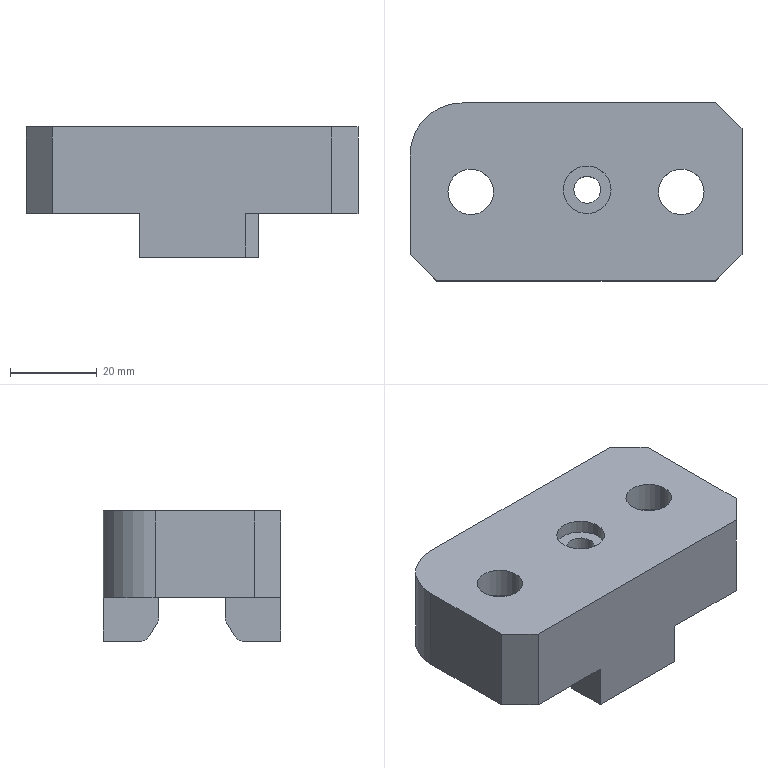Part | STEP file | lll_id2726_x_t | 1 solid | 35 faces | box 76.5 x 41 x 30 mm | volume 58200 mm3 | plane 24 | cylinder 11 | commonest cylinder face diameters 4 x4 10.5 x2 19.007 x2 6.2 x1 11 x1 24 x1
STEP:
#1=CARTESIAN_POINT('',(3745.164,7.62,-2.113));
#2=VERTEX_POINT('',#1);
#3=CARTESIAN_POINT('',(3772.5,7.62,-2.113));
#4=VERTEX_POINT('',#3);
#5=CARTESIAN_POINT('',(3772.5,7.62,-2.113));
#6=DIRECTION('',(1.,0.,0.));
#7=VECTOR('',#6,1.);
#8=LINE('',#5,#7);
#9=EDGE_CURVE('',#2,#4,#8,.T.);
#10=ORIENTED_EDGE('',*,*,#9,.F.);
#11=CARTESIAN_POINT('',(3745.164,7.905,-3.142));
#12=VERTEX_POINT('',#11);
#13=CARTESIAN_POINT('',(3745.164,9.62,-2.113));
#14=DIRECTION('',(1.,0.,0.));
#15=DIRECTION('',(0.,0.,-1.));
#16=AXIS2_PLACEMENT_3D('',#13,#14,#15);
#17=CIRCLE('',#16,2.);
#18=EDGE_CURVE('',#2,#12,#17,.T.);
#19=ORIENTED_EDGE('',*,*,#18,.T.);
#20=CARTESIAN_POINT('',(3772.5,7.905,-3.142));
#21=VERTEX_POINT('',#20);
#22=CARTESIAN_POINT('',(3758.811,7.905,-3.142));
#23=DIRECTION('',(-1.,0.,0.));
#24=VECTOR('',#23,1.);
#25=LINE('',#22,#24);
#26=EDGE_CURVE('',#21,#12,#25,.T.);
#27=ORIENTED_EDGE('',*,*,#26,.F.);
#28=CARTESIAN_POINT('',(3772.5,9.62,-2.113));
#29=DIRECTION('',(1.,0.,0.));
#30=DIRECTION('',(0.,0.,-1.));
#31=AXIS2_PLACEMENT_3D('',#28,#29,#30);
#32=CIRCLE('',#31,2.);
#33=EDGE_CURVE('',#4,#21,#32,.T.);
#34=ORIENTED_EDGE('',*,*,#33,.F.);
#35=EDGE_LOOP('',(#10,#19,#27,#34));
#36=FACE_OUTER_BOUND('',#35,.T.);
#37=CARTESIAN_POINT('',(3831.,9.62,-2.113));
#38=DIRECTION('',(1.,0.,0.));
#39=DIRECTION('',(0.,1.,0.));
#40=AXIS2_PLACEMENT_3D('',#37,#38,#39);
#41=CYLINDRICAL_SURFACE('',#40,2.);
#42=ADVANCED_FACE('',(#36),#41,.T.);
#43=CARTESIAN_POINT('',(3745.164,-7.62,-2.113));
#44=VERTEX_POINT('',#43);
#45=CARTESIAN_POINT('',(3745.164,-7.905,-3.142));
#46=VERTEX_POINT('',#45);
#47=CARTESIAN_POINT('',(3745.164,-9.62,-2.113));
#48=DIRECTION('',(-1.,0.,0.));
#49=DIRECTION('',(0.,0.,-1.));
#50=AXIS2_PLACEMENT_3D('',#47,#48,#49);
#51=CIRCLE('',#50,2.);
#52=EDGE_CURVE('',#44,#46,#51,.T.);
#53=ORIENTED_EDGE('',*,*,#52,.F.);
#54=CARTESIAN_POINT('',(3772.5,-7.62,-2.113));
#55=VERTEX_POINT('',#54);
#56=CARTESIAN_POINT('',(3758.811,-7.62,-2.113));
#57=DIRECTION('',(-1.,0.,0.));
#58=VECTOR('',#57,1.);
#59=LINE('',#56,#58);
#60=EDGE_CURVE('',#55,#44,#59,.T.);
#61=ORIENTED_EDGE('',*,*,#60,.F.);
#62=CARTESIAN_POINT('',(3772.5,-7.905,-3.142));
#63=VERTEX_POINT('',#62);
#64=CARTESIAN_POINT('',(3772.5,-9.62,-2.113));
#65=DIRECTION('',(1.,0.,0.));
#66=DIRECTION('',(0.,0.,-1.));
#67=AXIS2_PLACEMENT_3D('',#64,#65,#66);
#68=CIRCLE('',#67,2.);
#69=EDGE_CURVE('',#63,#55,#68,.T.);
#70=ORIENTED_EDGE('',*,*,#69,.F.);
#71=CARTESIAN_POINT('',(3772.5,-7.905,-3.142));
#72=DIRECTION('',(1.,0.,0.));
#73=VECTOR('',#72,1.);
#74=LINE('',#71,#73);
#75=EDGE_CURVE('',#46,#63,#74,.T.);
#76=ORIENTED_EDGE('',*,*,#75,.F.);
#77=EDGE_LOOP('',(#53,#61,#70,#76));
#78=FACE_OUTER_BOUND('',#77,.T.);
#79=CARTESIAN_POINT('',(3831.,-9.62,-2.113));
#80=DIRECTION('',(-1.,0.,0.));
#81=DIRECTION('',(0.,-1.,0.));
#82=AXIS2_PLACEMENT_3D('',#79,#80,#81);
#83=CYLINDRICAL_SURFACE('',#82,2.);
#84=ADVANCED_FACE('',(#78),#83,.T.);
#85=CARTESIAN_POINT('',(3772.5,-9.937,-6.529));
#86=VERTEX_POINT('',#85);
#87=CARTESIAN_POINT('',(3772.5,1.088,11.847));
#88=DIRECTION('',(0.,0.5145,0.8575));
#89=VECTOR('',#88,1.);
#90=LINE('',#87,#89);
#91=EDGE_CURVE('',#86,#63,#90,.T.);
#92=ORIENTED_EDGE('',*,*,#91,.T.);
#93=ORIENTED_EDGE('',*,*,#69,.T.);
#94=CARTESIAN_POINT('',(3772.5,-7.62,2.5));
#95=VERTEX_POINT('',#94);
#96=CARTESIAN_POINT('',(3772.5,-7.62,12.5));
#97=DIRECTION('',(0.,0.,-1.));
#98=VECTOR('',#97,1.);
#99=LINE('',#96,#98);
#100=EDGE_CURVE('',#95,#55,#99,.T.);
#101=ORIENTED_EDGE('',*,*,#100,.F.);
#102=CARTESIAN_POINT('',(3772.5,-17.5,2.5));
#103=VERTEX_POINT('',#102);
#104=CARTESIAN_POINT('',(3772.5,0.00007422,2.5));
#105=DIRECTION('',(0.,-1.,0.));
#106=VECTOR('',#105,1.);
#107=LINE('',#104,#106);
#108=EDGE_CURVE('',#95,#103,#107,.T.);
#109=ORIENTED_EDGE('',*,*,#108,.T.);
#110=CARTESIAN_POINT('',(3772.5,-17.5,-7.5));
#111=VERTEX_POINT('',#110);
#112=CARTESIAN_POINT('',(3772.5,-17.5,-7.5));
#113=DIRECTION('',(0.,0.,-1.));
#114=VECTOR('',#113,1.);
#115=LINE('',#112,#114);
#116=EDGE_CURVE('',#103,#111,#115,.T.);
#117=ORIENTED_EDGE('',*,*,#116,.T.);
#118=CARTESIAN_POINT('',(3772.5,-11.652,-7.5));
#119=VERTEX_POINT('',#118);
#120=CARTESIAN_POINT('',(3772.5,1.,-7.5));
#121=DIRECTION('',(0.,1.,0.));
#122=VECTOR('',#121,1.);
#123=LINE('',#120,#122);
#124=EDGE_CURVE('',#111,#119,#123,.T.);
#125=ORIENTED_EDGE('',*,*,#124,.T.);
#126=CARTESIAN_POINT('',(3772.5,-11.652,-5.5));
#127=DIRECTION('',(1.,0.,0.));
#128=DIRECTION('',(0.,0.,-1.));
#129=AXIS2_PLACEMENT_3D('',#126,#127,#128);
#130=CIRCLE('',#129,2.);
#131=EDGE_CURVE('',#119,#86,#130,.T.);
#132=ORIENTED_EDGE('',*,*,#131,.T.);
#133=EDGE_LOOP('',(#92,#93,#101,#109,#117,#125,#132));
#134=FACE_OUTER_BOUND('',#133,.T.);
#135=CARTESIAN_POINT('',(3772.5,0.00007422,12.5));
#136=DIRECTION('',(1.,0.,0.));
#137=DIRECTION('',(0.,0.,-1.));
#138=AXIS2_PLACEMENT_3D('',#135,#136,#137);
#139=PLANE('',#138);
#140=ADVANCED_FACE('',(#134),#139,.T.);
#141=CARTESIAN_POINT('',(3772.5,7.62,2.5));
#142=VERTEX_POINT('',#141);
#143=CARTESIAN_POINT('',(3772.5,7.62,12.5));
#144=DIRECTION('',(0.,0.,-1.));
#145=VECTOR('',#144,1.);
#146=LINE('',#143,#145);
#147=EDGE_CURVE('',#142,#4,#146,.T.);
#148=ORIENTED_EDGE('',*,*,#147,.T.);
#149=ORIENTED_EDGE('',*,*,#33,.T.);
#150=CARTESIAN_POINT('',(3772.5,9.937,-6.529));
#151=VERTEX_POINT('',#150);
#152=CARTESIAN_POINT('',(3772.5,-1.088,11.847));
#153=DIRECTION('',(0.,0.5145,-0.8575));
#154=VECTOR('',#153,1.);
#155=LINE('',#152,#154);
#156=EDGE_CURVE('',#21,#151,#155,.T.);
#157=ORIENTED_EDGE('',*,*,#156,.T.);
#158=CARTESIAN_POINT('',(3772.5,11.652,-7.5));
#159=VERTEX_POINT('',#158);
#160=CARTESIAN_POINT('',(3772.5,11.652,-5.5));
#161=DIRECTION('',(1.,0.,0.));
#162=DIRECTION('',(0.,0.,-1.));
#163=AXIS2_PLACEMENT_3D('',#160,#161,#162);
#164=CIRCLE('',#163,2.);
#165=EDGE_CURVE('',#151,#159,#164,.T.);
#166=ORIENTED_EDGE('',*,*,#165,.T.);
#167=CARTESIAN_POINT('',(3772.5,17.5,-7.5));
#168=VERTEX_POINT('',#167);
#169=CARTESIAN_POINT('',(3772.5,-0.9999,-7.5));
#170=DIRECTION('',(0.,1.,0.));
#171=VECTOR('',#170,1.);
#172=LINE('',#169,#171);
#173=EDGE_CURVE('',#159,#168,#172,.T.);
#174=ORIENTED_EDGE('',*,*,#173,.T.);
#175=CARTESIAN_POINT('',(3772.5,17.5,2.5));
#176=VERTEX_POINT('',#175);
#177=CARTESIAN_POINT('',(3772.5,17.5,2.5));
#178=DIRECTION('',(0.,0.,1.));
#179=VECTOR('',#178,1.);
#180=LINE('',#177,#179);
#181=EDGE_CURVE('',#168,#176,#180,.T.);
#182=ORIENTED_EDGE('',*,*,#181,.T.);
#183=CARTESIAN_POINT('',(3772.5,0.00007422,2.5));
#184=DIRECTION('',(0.,-1.,0.));
#185=VECTOR('',#184,1.);
#186=LINE('',#183,#185);
#187=EDGE_CURVE('',#176,#142,#186,.T.);
#188=ORIENTED_EDGE('',*,*,#187,.T.);
#189=EDGE_LOOP('',(#148,#149,#157,#166,#174,#182,#188));
#190=FACE_OUTER_BOUND('',#189,.T.);
#191=CARTESIAN_POINT('',(3772.5,0.00007422,12.5));
#192=DIRECTION('',(1.,0.,0.));
#193=DIRECTION('',(0.,0.,-1.));
#194=AXIS2_PLACEMENT_3D('',#191,#192,#193);
#195=PLANE('',#194);
#196=ADVANCED_FACE('',(#190),#195,.T.);
#197=CARTESIAN_POINT('',(3771.997,0.00007422,15.5));
#198=VERTEX_POINT('',#197);
#199=CARTESIAN_POINT('',(3781.5,0.00007422,15.5));
#200=DIRECTION('',(0.,0.,1.));
#201=DIRECTION('',(-1.,0.,0.));
#202=AXIS2_PLACEMENT_3D('',#199,#200,#201);
#203=CIRCLE('',#202,9.504);
#204=EDGE_CURVE('',#198,#198,#203,.T.);
#205=ORIENTED_EDGE('',*,*,#204,.F.);
#206=EDGE_LOOP('',(#205));
#207=FACE_BOUND('',#206,.T.);
#208=CARTESIAN_POINT('',(3776.25,0.00007422,15.5));
#209=VERTEX_POINT('',#208);
#210=CARTESIAN_POINT('',(3781.5,0.00007422,15.5));
#211=DIRECTION('',(0.,0.,1.));
#212=DIRECTION('',(-1.,0.,0.));
#213=AXIS2_PLACEMENT_3D('',#210,#211,#212);
#214=CIRCLE('',#213,5.25);
#215=EDGE_CURVE('',#209,#209,#214,.T.);
#216=ORIENTED_EDGE('',*,*,#215,.T.);
#217=EDGE_LOOP('',(#216));
#218=FACE_BOUND('',#217,.T.);
#219=CARTESIAN_POINT('',(3781.5,0.00007422,15.5));
#220=DIRECTION('',(0.,0.,1.));
#221=DIRECTION('',(-1.,0.,0.));
#222=AXIS2_PLACEMENT_3D('',#219,#220,#221);
#223=PLANE('',#222);
#224=ADVANCED_FACE('',(#207,#218),#223,.F.);
#225=CARTESIAN_POINT('',(3775.5,7.37,2.5));
#226=VERTEX_POINT('',#225);
#227=CARTESIAN_POINT('',(3781.5,0.00007422,2.5));
#228=DIRECTION('',(0.,0.,1.));
#229=DIRECTION('',(1.,0.,0.));
#230=AXIS2_PLACEMENT_3D('',#227,#228,#229);
#231=CIRCLE('',#230,9.504);
#232=EDGE_CURVE('',#226,#226,#231,.T.);
#233=ORIENTED_EDGE('',*,*,#232,.F.);
#234=EDGE_LOOP('',(#233));
#235=FACE_BOUND('',#234,.T.);
#236=ORIENTED_EDGE('',*,*,#204,.T.);
#237=EDGE_LOOP('',(#236));
#238=FACE_BOUND('',#237,.T.);
#239=CARTESIAN_POINT('',(3781.5,0.00007422,2.5));
#240=DIRECTION('',(0.,0.,1.));
#241=DIRECTION('',(-1.,0.,0.));
#242=AXIS2_PLACEMENT_3D('',#239,#240,#241);
#243=CYLINDRICAL_SURFACE('',#242,9.504);
#244=ADVANCED_FACE('',(#235,#238),#243,.F.);
#245=CARTESIAN_POINT('',(3745.164,11.652,-7.5));
#246=VERTEX_POINT('',#245);
#247=CARTESIAN_POINT('',(3759.758,11.652,-7.5));
#248=DIRECTION('',(-1.,0.,0.));
#249=VECTOR('',#248,1.);
#250=LINE('',#247,#249);
#251=EDGE_CURVE('',#159,#246,#250,.T.);
#252=ORIENTED_EDGE('',*,*,#251,.T.);
#253=CARTESIAN_POINT('',(3745.164,20.5,-7.5));
#254=VERTEX_POINT('',#253);
#255=CARTESIAN_POINT('',(3745.164,-0.9999,-7.5));
#256=DIRECTION('',(0.,1.,0.));
#257=VECTOR('',#256,1.);
#258=LINE('',#255,#257);
#259=EDGE_CURVE('',#246,#254,#258,.T.);
#260=ORIENTED_EDGE('',*,*,#259,.T.);
#261=CARTESIAN_POINT('',(3769.5,20.5,-7.5));
#262=VERTEX_POINT('',#261);
#263=CARTESIAN_POINT('',(7344.751,20.5,-7.5));
#264=DIRECTION('',(1.,0.,0.));
#265=VECTOR('',#264,1.);
#266=LINE('',#263,#265);
#267=EDGE_CURVE('',#254,#262,#266,.T.);
#268=ORIENTED_EDGE('',*,*,#267,.T.);
#269=CARTESIAN_POINT('',(3772.5,17.5,-7.5));
#270=DIRECTION('',(0.7071,-0.7071,0.));
#271=VECTOR('',#270,1.);
#272=LINE('',#269,#271);
#273=EDGE_CURVE('',#262,#168,#272,.T.);
#274=ORIENTED_EDGE('',*,*,#273,.T.);
#275=ORIENTED_EDGE('',*,*,#173,.F.);
#276=EDGE_LOOP('',(#252,#260,#268,#274,#275));
#277=FACE_OUTER_BOUND('',#276,.T.);
#278=CARTESIAN_POINT('',(7344.751,-0.9999,-7.5));
#279=DIRECTION('',(0.,0.,1.));
#280=DIRECTION('',(1.,0.,0.));
#281=AXIS2_PLACEMENT_3D('',#278,#279,#280);
#282=PLANE('',#281);
#283=ADVANCED_FACE('',(#277),#282,.F.);
#284=CARTESIAN_POINT('',(3745.164,-20.5,-7.5));
#285=VERTEX_POINT('',#284);
#286=CARTESIAN_POINT('',(3745.164,-11.652,-7.5));
#287=VERTEX_POINT('',#286);
#288=CARTESIAN_POINT('',(3745.164,1.,-7.5));
#289=DIRECTION('',(0.,1.,0.));
#290=VECTOR('',#289,1.);
#291=LINE('',#288,#290);
#292=EDGE_CURVE('',#285,#287,#291,.T.);
#293=ORIENTED_EDGE('',*,*,#292,.T.);
#294=CARTESIAN_POINT('',(3772.5,-11.652,-7.5));
#295=DIRECTION('',(1.,0.,0.));
#296=VECTOR('',#295,1.);
#297=LINE('',#294,#296);
#298=EDGE_CURVE('',#287,#119,#297,.T.);
#299=ORIENTED_EDGE('',*,*,#298,.T.);
#300=ORIENTED_EDGE('',*,*,#124,.F.);
#301=CARTESIAN_POINT('',(3769.5,-20.5,-7.5));
#302=VERTEX_POINT('',#301);
#303=CARTESIAN_POINT('',(3769.5,-20.5,-7.5));
#304=DIRECTION('',(-0.7071,-0.7071,0.));
#305=VECTOR('',#304,1.);
#306=LINE('',#303,#305);
#307=EDGE_CURVE('',#111,#302,#306,.T.);
#308=ORIENTED_EDGE('',*,*,#307,.T.);
#309=CARTESIAN_POINT('',(3794.,-20.5,-7.5));
#310=DIRECTION('',(1.,0.,0.));
#311=VECTOR('',#310,1.);
#312=LINE('',#309,#311);
#313=EDGE_CURVE('',#285,#302,#312,.T.);
#314=ORIENTED_EDGE('',*,*,#313,.F.);
#315=EDGE_LOOP('',(#293,#299,#300,#308,#314));
#316=FACE_OUTER_BOUND('',#315,.T.);
#317=CARTESIAN_POINT('',(7344.751,1.,-7.5));
#318=DIRECTION('',(0.,0.,1.));
#319=DIRECTION('',(1.,0.,0.));
#320=AXIS2_PLACEMENT_3D('',#317,#318,#319);
#321=PLANE('',#320);
#322=ADVANCED_FACE('',(#316),#321,.F.);
#323=CARTESIAN_POINT('',(3745.164,20.5,2.5));
#324=VERTEX_POINT('',#323);
#325=CARTESIAN_POINT('',(3731.,20.5,2.5));
#326=VERTEX_POINT('',#325);
#327=CARTESIAN_POINT('',(3794.,20.5,2.5));
#328=DIRECTION('',(-1.,0.,0.));
#329=VECTOR('',#328,1.);
#330=LINE('',#327,#329);
#331=EDGE_CURVE('',#324,#326,#330,.T.);
#332=ORIENTED_EDGE('',*,*,#331,.T.);
#333=CARTESIAN_POINT('',(3731.,20.5,22.5));
#334=VERTEX_POINT('',#333);
#335=CARTESIAN_POINT('',(3731.,20.5,12.5));
#336=DIRECTION('',(0.,0.,1.));
#337=VECTOR('',#336,1.);
#338=LINE('',#335,#337);
#339=EDGE_CURVE('',#326,#334,#338,.T.);
#340=ORIENTED_EDGE('',*,*,#339,.T.);
#341=CARTESIAN_POINT('',(3789.5,20.5,22.5));
#342=VERTEX_POINT('',#341);
#343=CARTESIAN_POINT('',(3774.,20.5,22.5));
#344=DIRECTION('',(-1.,0.,0.));
#345=VECTOR('',#344,1.);
#346=LINE('',#343,#345);
#347=EDGE_CURVE('',#342,#334,#346,.T.);
#348=ORIENTED_EDGE('',*,*,#347,.F.);
#349=CARTESIAN_POINT('',(3789.5,20.5,2.5));
#350=VERTEX_POINT('',#349);
#351=CARTESIAN_POINT('',(3789.5,20.5,12.5));
#352=DIRECTION('',(0.,0.,-1.));
#353=VECTOR('',#352,1.);
#354=LINE('',#351,#353);
#355=EDGE_CURVE('',#342,#350,#354,.T.);
#356=ORIENTED_EDGE('',*,*,#355,.T.);
#357=CARTESIAN_POINT('',(3769.5,20.5,2.5));
#358=VERTEX_POINT('',#357);
#359=CARTESIAN_POINT('',(3794.,20.5,2.5));
#360=DIRECTION('',(-1.,0.,0.));
#361=VECTOR('',#360,1.);
#362=LINE('',#359,#361);
#363=EDGE_CURVE('',#350,#358,#362,.T.);
#364=ORIENTED_EDGE('',*,*,#363,.T.);
#365=CARTESIAN_POINT('',(3769.5,20.5,-7.5));
#366=DIRECTION('',(0.,0.,-1.));
#367=VECTOR('',#366,1.);
#368=LINE('',#365,#367);
#369=EDGE_CURVE('',#358,#262,#368,.T.);
#370=ORIENTED_EDGE('',*,*,#369,.T.);
#371=ORIENTED_EDGE('',*,*,#267,.F.);
#372=CARTESIAN_POINT('',(3745.164,20.5,12.5));
#373=DIRECTION('',(0.,0.,1.));
#374=VECTOR('',#373,1.);
#375=LINE('',#372,#374);
#376=EDGE_CURVE('',#254,#324,#375,.T.);
#377=ORIENTED_EDGE('',*,*,#376,.T.);
#378=EDGE_LOOP('',(#332,#340,#348,#356,#364,#370,#371,#377));
#379=FACE_OUTER_BOUND('',#378,.T.);
#380=CARTESIAN_POINT('',(3794.,20.5,12.5));
#381=DIRECTION('',(0.,-1.,0.));
#382=DIRECTION('',(0.,0.,1.));
#383=AXIS2_PLACEMENT_3D('',#380,#381,#382);
#384=PLANE('',#383);
#385=ADVANCED_FACE('',(#379),#384,.F.);
#386=CARTESIAN_POINT('',(3789.5,-20.5,22.5));
#387=VERTEX_POINT('',#386);
#388=CARTESIAN_POINT('',(3725.,-20.5,22.5));
#389=VERTEX_POINT('',#388);
#390=CARTESIAN_POINT('',(3794.,-20.5,22.5));
#391=DIRECTION('',(-1.,0.,0.));
#392=VECTOR('',#391,1.);
#393=LINE('',#390,#392);
#394=EDGE_CURVE('',#387,#389,#393,.T.);
#395=ORIENTED_EDGE('',*,*,#394,.T.);
#396=CARTESIAN_POINT('',(3725.,-20.5,2.5));
#397=VERTEX_POINT('',#396);
#398=CARTESIAN_POINT('',(3725.,-20.5,12.5));
#399=DIRECTION('',(0.,0.,-1.));
#400=VECTOR('',#399,1.);
#401=LINE('',#398,#400);
#402=EDGE_CURVE('',#389,#397,#401,.T.);
#403=ORIENTED_EDGE('',*,*,#402,.T.);
#404=CARTESIAN_POINT('',(3745.164,-20.5,2.5));
#405=VERTEX_POINT('',#404);
#406=CARTESIAN_POINT('',(3794.,-20.5,2.5));
#407=DIRECTION('',(1.,0.,0.));
#408=VECTOR('',#407,1.);
#409=LINE('',#406,#408);
#410=EDGE_CURVE('',#397,#405,#409,.T.);
#411=ORIENTED_EDGE('',*,*,#410,.T.);
#412=CARTESIAN_POINT('',(3745.164,-20.5,12.5));
#413=DIRECTION('',(0.,0.,-1.));
#414=VECTOR('',#413,1.);
#415=LINE('',#412,#414);
#416=EDGE_CURVE('',#405,#285,#415,.T.);
#417=ORIENTED_EDGE('',*,*,#416,.T.);
#418=ORIENTED_EDGE('',*,*,#313,.T.);
#419=CARTESIAN_POINT('',(3769.5,-20.5,2.5));
#420=VERTEX_POINT('',#419);
#421=CARTESIAN_POINT('',(3769.5,-20.5,2.5));
#422=DIRECTION('',(0.,0.,1.));
#423=VECTOR('',#422,1.);
#424=LINE('',#421,#423);
#425=EDGE_CURVE('',#302,#420,#424,.T.);
#426=ORIENTED_EDGE('',*,*,#425,.T.);
#427=CARTESIAN_POINT('',(3789.5,-20.5,2.5));
#428=VERTEX_POINT('',#427);
#429=CARTESIAN_POINT('',(3794.,-20.5,2.5));
#430=DIRECTION('',(1.,0.,0.));
#431=VECTOR('',#430,1.);
#432=LINE('',#429,#431);
#433=EDGE_CURVE('',#420,#428,#432,.T.);
#434=ORIENTED_EDGE('',*,*,#433,.T.);
#435=CARTESIAN_POINT('',(3789.5,-20.5,12.5));
#436=DIRECTION('',(0.,0.,1.));
#437=VECTOR('',#436,1.);
#438=LINE('',#435,#437);
#439=EDGE_CURVE('',#428,#387,#438,.T.);
#440=ORIENTED_EDGE('',*,*,#439,.T.);
#441=EDGE_LOOP('',(#395,#403,#411,#417,#418,#426,#434,#440));
#442=FACE_OUTER_BOUND('',#441,.T.);
#443=CARTESIAN_POINT('',(3794.,-20.5,12.5));
#444=DIRECTION('',(0.,1.,0.));
#445=DIRECTION('',(0.,0.,1.));
#446=AXIS2_PLACEMENT_3D('',#443,#444,#445);
#447=PLANE('',#446);
#448=ADVANCED_FACE('',(#442),#447,.F.);
#449=CARTESIAN_POINT('',(3754.332,0.5,22.5));
#450=VERTEX_POINT('',#449);
#451=CARTESIAN_POINT('',(3759.832,0.5,22.5));
#452=DIRECTION('',(0.,0.,-1.));
#453=DIRECTION('',(-1.,0.,0.));
#454=AXIS2_PLACEMENT_3D('',#451,#452,#453);
#455=CIRCLE('',#454,5.5);
#456=EDGE_CURVE('',#450,#450,#455,.T.);
#457=ORIENTED_EDGE('',*,*,#456,.T.);
#458=EDGE_LOOP('',(#457));
#459=FACE_BOUND('',#458,.T.);
#460=CARTESIAN_POINT('',(3727.75,0.00007422,22.5));
#461=VERTEX_POINT('',#460);
#462=CARTESIAN_POINT('',(3733.,0.00007422,22.5));
#463=DIRECTION('',(0.,0.,-1.));
#464=DIRECTION('',(-1.,0.,0.));
#465=AXIS2_PLACEMENT_3D('',#462,#463,#464);
#466=CIRCLE('',#465,5.25);
#467=EDGE_CURVE('',#461,#461,#466,.T.);
#468=ORIENTED_EDGE('',*,*,#467,.T.);
#469=EDGE_LOOP('',(#468));
#470=FACE_BOUND('',#469,.T.);
#471=ORIENTED_EDGE('',*,*,#347,.T.);
#472=CARTESIAN_POINT('',(3719.,8.5,22.5));
#473=VERTEX_POINT('',#472);
#474=CARTESIAN_POINT('',(3731.,8.5,22.5));
#475=DIRECTION('',(0.,0.,1.));
#476=DIRECTION('',(-1.,0.,0.));
#477=AXIS2_PLACEMENT_3D('',#474,#475,#476);
#478=CIRCLE('',#477,12.);
#479=EDGE_CURVE('',#334,#473,#478,.T.);
#480=ORIENTED_EDGE('',*,*,#479,.T.);
#481=CARTESIAN_POINT('',(3719.,-14.5,22.5));
#482=VERTEX_POINT('',#481);
#483=CARTESIAN_POINT('',(3719.,40.,22.5));
#484=DIRECTION('',(0.,-1.,0.));
#485=VECTOR('',#484,1.);
#486=LINE('',#483,#485);
#487=EDGE_CURVE('',#473,#482,#486,.T.);
#488=ORIENTED_EDGE('',*,*,#487,.T.);
#489=CARTESIAN_POINT('',(3719.,-14.5,22.5));
#490=DIRECTION('',(0.7071,-0.7071,0.));
#491=VECTOR('',#490,1.);
#492=LINE('',#489,#491);
#493=EDGE_CURVE('',#482,#389,#492,.T.);
#494=ORIENTED_EDGE('',*,*,#493,.T.);
#495=ORIENTED_EDGE('',*,*,#394,.F.);
#496=CARTESIAN_POINT('',(3795.5,-14.5,22.5));
#497=VERTEX_POINT('',#496);
#498=CARTESIAN_POINT('',(3789.5,-20.5,22.5));
#499=DIRECTION('',(0.7071,0.7071,0.));
#500=VECTOR('',#499,1.);
#501=LINE('',#498,#500);
#502=EDGE_CURVE('',#387,#497,#501,.T.);
#503=ORIENTED_EDGE('',*,*,#502,.T.);
#504=CARTESIAN_POINT('',(3795.5,14.5,22.5));
#505=VERTEX_POINT('',#504);
#506=CARTESIAN_POINT('',(3795.5,40.,22.5));
#507=DIRECTION('',(0.,-1.,0.));
#508=VECTOR('',#507,1.);
#509=LINE('',#506,#508);
#510=EDGE_CURVE('',#505,#497,#509,.T.);
#511=ORIENTED_EDGE('',*,*,#510,.F.);
#512=CARTESIAN_POINT('',(3789.5,20.5,22.5));
#513=DIRECTION('',(-0.7071,0.7071,0.));
#514=VECTOR('',#513,1.);
#515=LINE('',#512,#514);
#516=EDGE_CURVE('',#505,#342,#515,.T.);
#517=ORIENTED_EDGE('',*,*,#516,.T.);
#518=EDGE_LOOP('',(#471,#480,#488,#494,#495,#503,#511,#517));
#519=FACE_BOUND('',#518,.T.);
#520=CARTESIAN_POINT('',(3776.25,0.00007422,22.5));
#521=VERTEX_POINT('',#520);
#522=CARTESIAN_POINT('',(3781.5,0.00007422,22.5));
#523=DIRECTION('',(0.,0.,-1.));
#524=DIRECTION('',(-1.,0.,0.));
#525=AXIS2_PLACEMENT_3D('',#522,#523,#524);
#526=CIRCLE('',#525,5.25);
#527=EDGE_CURVE('',#521,#521,#526,.T.);
#528=ORIENTED_EDGE('',*,*,#527,.T.);
#529=EDGE_LOOP('',(#528));
#530=FACE_BOUND('',#529,.T.);
#531=CARTESIAN_POINT('',(3774.,40.,22.5));
#532=DIRECTION('',(0.,0.,-1.));
#533=DIRECTION('',(-1.,0.,0.));
#534=AXIS2_PLACEMENT_3D('',#531,#532,#533);
#535=PLANE('',#534);
#536=ADVANCED_FACE('',(#459,#470,#519,#530),#535,.F.);
#537=CARTESIAN_POINT('',(3745.164,7.62,2.5));
#538=VERTEX_POINT('',#537);
#539=CARTESIAN_POINT('',(3745.164,7.62,2.5));
#540=DIRECTION('',(0.,0.,1.));
#541=VECTOR('',#540,1.);
#542=LINE('',#539,#541);
#543=EDGE_CURVE('',#2,#538,#542,.T.);
#544=ORIENTED_EDGE('',*,*,#543,.F.);
#545=ORIENTED_EDGE('',*,*,#9,.T.);
#546=ORIENTED_EDGE('',*,*,#147,.F.);
#547=CARTESIAN_POINT('',(3774.,7.62,2.5));
#548=DIRECTION('',(1.,0.,0.));
#549=VECTOR('',#548,1.);
#550=LINE('',#547,#549);
#551=EDGE_CURVE('',#538,#142,#550,.T.);
#552=ORIENTED_EDGE('',*,*,#551,.F.);
#553=EDGE_LOOP('',(#544,#545,#546,#552));
#554=FACE_OUTER_BOUND('',#553,.T.);
#555=CARTESIAN_POINT('',(3831.,7.62,2.5));
#556=DIRECTION('',(0.,-1.,0.));
#557=DIRECTION('',(-1.,0.,0.));
#558=AXIS2_PLACEMENT_3D('',#555,#556,#557);
#559=PLANE('',#558);
#560=ADVANCED_FACE('',(#554),#559,.T.);
#561=CARTESIAN_POINT('',(3762.932,0.5,2.5));
#562=VERTEX_POINT('',#561);
#563=CARTESIAN_POINT('',(3759.832,0.5,2.5));
#564=DIRECTION('',(0.,0.,1.));
#565=DIRECTION('',(1.,0.,0.));
#566=AXIS2_PLACEMENT_3D('',#563,#564,#565);
#567=CIRCLE('',#566,3.1);
#568=EDGE_CURVE('',#562,#562,#567,.T.);
#569=ORIENTED_EDGE('',*,*,#568,.T.);
#570=EDGE_LOOP('',(#569));
#571=FACE_BOUND('',#570,.T.);
#572=CARTESIAN_POINT('',(3719.,-14.5,2.5));
#573=VERTEX_POINT('',#572);
#574=CARTESIAN_POINT('',(3719.,8.5,2.5));
#575=VERTEX_POINT('',#574);
#576=CARTESIAN_POINT('',(3719.,-26.737,2.5));
#577=DIRECTION('',(0.,1.,0.));
#578=VECTOR('',#577,1.);
#579=LINE('',#576,#578);
#580=EDGE_CURVE('',#573,#575,#579,.T.);
#581=ORIENTED_EDGE('',*,*,#580,.T.);
#582=CARTESIAN_POINT('',(3731.,8.5,2.5));
#583=DIRECTION('',(0.,0.,-1.));
#584=DIRECTION('',(1.,0.,0.));
#585=AXIS2_PLACEMENT_3D('',#582,#583,#584);
#586=CIRCLE('',#585,12.);
#587=EDGE_CURVE('',#575,#326,#586,.T.);
#588=ORIENTED_EDGE('',*,*,#587,.T.);
#589=ORIENTED_EDGE('',*,*,#331,.F.);
#590=CARTESIAN_POINT('',(3745.164,-3.5,2.5));
#591=DIRECTION('',(0.,-1.,0.));
#592=VECTOR('',#591,1.);
#593=LINE('',#590,#592);
#594=EDGE_CURVE('',#324,#538,#593,.T.);
#595=ORIENTED_EDGE('',*,*,#594,.T.);
#596=ORIENTED_EDGE('',*,*,#551,.T.);
#597=ORIENTED_EDGE('',*,*,#187,.F.);
#598=CARTESIAN_POINT('',(3795.369,-5.368,2.5));
#599=DIRECTION('',(-0.7071,0.7071,0.));
#600=VECTOR('',#599,1.);
#601=LINE('',#598,#600);
#602=EDGE_CURVE('',#176,#358,#601,.T.);
#603=ORIENTED_EDGE('',*,*,#602,.T.);
#604=ORIENTED_EDGE('',*,*,#363,.F.);
#605=CARTESIAN_POINT('',(3795.5,14.5,2.5));
#606=VERTEX_POINT('',#605);
#607=CARTESIAN_POINT('',(3789.5,20.5,2.5));
#608=DIRECTION('',(0.7071,-0.7071,0.));
#609=VECTOR('',#608,1.);
#610=LINE('',#607,#609);
#611=EDGE_CURVE('',#350,#606,#610,.T.);
#612=ORIENTED_EDGE('',*,*,#611,.T.);
#613=CARTESIAN_POINT('',(3795.5,-14.5,2.5));
#614=VERTEX_POINT('',#613);
#615=CARTESIAN_POINT('',(3795.5,-26.737,2.5));
#616=DIRECTION('',(0.,-1.,0.));
#617=VECTOR('',#616,1.);
#618=LINE('',#615,#617);
#619=EDGE_CURVE('',#606,#614,#618,.T.);
#620=ORIENTED_EDGE('',*,*,#619,.T.);
#621=CARTESIAN_POINT('',(3789.5,-20.5,2.5));
#622=DIRECTION('',(-0.7071,-0.7071,0.));
#623=VECTOR('',#622,1.);
#624=LINE('',#621,#623);
#625=EDGE_CURVE('',#614,#428,#624,.T.);
#626=ORIENTED_EDGE('',*,*,#625,.T.);
#627=ORIENTED_EDGE('',*,*,#433,.F.);
#628=CARTESIAN_POINT('',(3768.632,-21.368,2.5));
#629=DIRECTION('',(0.7071,0.7071,0.));
#630=VECTOR('',#629,1.);
#631=LINE('',#628,#630);
#632=EDGE_CURVE('',#420,#103,#631,.T.);
#633=ORIENTED_EDGE('',*,*,#632,.T.);
#634=ORIENTED_EDGE('',*,*,#108,.F.);
#635=CARTESIAN_POINT('',(3745.164,-7.62,2.5));
#636=VERTEX_POINT('',#635);
#637=CARTESIAN_POINT('',(3774.,-7.62,2.5));
#638=DIRECTION('',(1.,0.,0.));
#639=VECTOR('',#638,1.);
#640=LINE('',#637,#639);
#641=EDGE_CURVE('',#636,#95,#640,.T.);
#642=ORIENTED_EDGE('',*,*,#641,.F.);
#643=CARTESIAN_POINT('',(3745.164,-3.5,2.5));
#644=DIRECTION('',(0.,-1.,0.));
#645=VECTOR('',#644,1.);
#646=LINE('',#643,#645);
#647=EDGE_CURVE('',#636,#405,#646,.T.);
#648=ORIENTED_EDGE('',*,*,#647,.T.);
#649=ORIENTED_EDGE('',*,*,#410,.F.);
#650=CARTESIAN_POINT('',(3719.,-14.5,2.5));
#651=DIRECTION('',(-0.7071,0.7071,0.));
#652=VECTOR('',#651,1.);
#653=LINE('',#650,#652);
#654=EDGE_CURVE('',#397,#573,#653,.T.);
#655=ORIENTED_EDGE('',*,*,#654,.T.);
#656=EDGE_LOOP('',(#581,#588,#589,#595,#596,#597,#603,#604,#612,#620,#626,#627,#633,#634,#642,#648,#649,#655));
#657=FACE_BOUND('',#656,.T.);
#658=CARTESIAN_POINT('',(3742.504,0.00007422,2.5));
#659=VERTEX_POINT('',#658);
#660=CARTESIAN_POINT('',(3733.,0.00007422,2.5));
#661=DIRECTION('',(0.,0.,1.));
#662=DIRECTION('',(1.,0.,0.));
#663=AXIS2_PLACEMENT_3D('',#660,#661,#662);
#664=CIRCLE('',#663,9.504);
#665=EDGE_CURVE('',#659,#659,#664,.T.);
#666=ORIENTED_EDGE('',*,*,#665,.T.);
#667=EDGE_LOOP('',(#666));
#668=FACE_BOUND('',#667,.T.);
#669=ORIENTED_EDGE('',*,*,#232,.T.);
#670=EDGE_LOOP('',(#669));
#671=FACE_BOUND('',#670,.T.);
#672=CARTESIAN_POINT('',(3774.,-26.737,2.5));
#673=DIRECTION('',(0.,0.,1.));
#674=DIRECTION('',(1.,0.,0.));
#675=AXIS2_PLACEMENT_3D('',#672,#673,#674);
#676=PLANE('',#675);
#677=ADVANCED_FACE('',(#571,#657,#668,#671),#676,.F.);
#678=CARTESIAN_POINT('',(3745.164,-7.62,-10.));
#679=DIRECTION('',(0.,0.,-1.));
#680=VECTOR('',#679,1.);
#681=LINE('',#678,#680);
#682=EDGE_CURVE('',#636,#44,#681,.T.);
#683=ORIENTED_EDGE('',*,*,#682,.F.);
#684=ORIENTED_EDGE('',*,*,#641,.T.);
#685=ORIENTED_EDGE('',*,*,#100,.T.);
#686=ORIENTED_EDGE('',*,*,#60,.T.);
#687=EDGE_LOOP('',(#683,#684,#685,#686));
#688=FACE_OUTER_BOUND('',#687,.T.);
#689=CARTESIAN_POINT('',(3831.,-7.62,2.5));
#690=DIRECTION('',(0.,-1.,0.));
#691=DIRECTION('',(-1.,0.,0.));
#692=AXIS2_PLACEMENT_3D('',#689,#690,#691);
#693=PLANE('',#692);
#694=ADVANCED_FACE('',(#688),#693,.F.);
#695=ORIENTED_EDGE('',*,*,#487,.F.);
#696=CARTESIAN_POINT('',(3719.,8.5,12.5));
#697=DIRECTION('',(0.,0.,-1.));
#698=VECTOR('',#697,1.);
#699=LINE('',#696,#698);
#700=EDGE_CURVE('',#473,#575,#699,.T.);
#701=ORIENTED_EDGE('',*,*,#700,.T.);
#702=ORIENTED_EDGE('',*,*,#580,.F.);
#703=CARTESIAN_POINT('',(3719.,-14.5,12.5));
#704=DIRECTION('',(0.,0.,1.));
#705=VECTOR('',#704,1.);
#706=LINE('',#703,#705);
#707=EDGE_CURVE('',#573,#482,#706,.T.);
#708=ORIENTED_EDGE('',*,*,#707,.T.);
#709=EDGE_LOOP('',(#695,#701,#702,#708));
#710=FACE_OUTER_BOUND('',#709,.T.);
#711=CARTESIAN_POINT('',(3719.,-26.737,12.5));
#712=DIRECTION('',(1.,0.,0.));
#713=DIRECTION('',(0.,0.,-1.));
#714=AXIS2_PLACEMENT_3D('',#711,#712,#713);
#715=PLANE('',#714);
#716=ADVANCED_FACE('',(#710),#715,.F.);
#717=CARTESIAN_POINT('',(3742.504,0.00007422,15.5));
#718=VERTEX_POINT('',#717);
#719=CARTESIAN_POINT('',(3733.,0.00007422,15.5));
#720=DIRECTION('',(0.,0.,1.));
#721=DIRECTION('',(1.,0.,0.));
#722=AXIS2_PLACEMENT_3D('',#719,#720,#721);
#723=CIRCLE('',#722,9.504);
#724=EDGE_CURVE('',#718,#718,#723,.T.);
#725=ORIENTED_EDGE('',*,*,#724,.F.);
#726=EDGE_LOOP('',(#725));
#727=FACE_BOUND('',#726,.T.);
#728=CARTESIAN_POINT('',(3738.25,0.00007422,15.5));
#729=VERTEX_POINT('',#728);
#730=CARTESIAN_POINT('',(3733.,0.00007422,15.5));
#731=DIRECTION('',(0.,0.,1.));
#732=DIRECTION('',(1.,0.,0.));
#733=AXIS2_PLACEMENT_3D('',#730,#731,#732);
#734=CIRCLE('',#733,5.25);
#735=EDGE_CURVE('',#729,#729,#734,.T.);
#736=ORIENTED_EDGE('',*,*,#735,.T.);
#737=EDGE_LOOP('',(#736));
#738=FACE_BOUND('',#737,.T.);
#739=CARTESIAN_POINT('',(3733.,0.00007422,15.5));
#740=DIRECTION('',(0.,0.,1.));
#741=DIRECTION('',(1.,0.,0.));
#742=AXIS2_PLACEMENT_3D('',#739,#740,#741);
#743=PLANE('',#742);
#744=ADVANCED_FACE('',(#727,#738),#743,.F.);
#745=ORIENTED_EDGE('',*,*,#665,.F.);
#746=EDGE_LOOP('',(#745));
#747=FACE_BOUND('',#746,.T.);
#748=ORIENTED_EDGE('',*,*,#724,.T.);
#749=EDGE_LOOP('',(#748));
#750=FACE_BOUND('',#749,.T.);
#751=CARTESIAN_POINT('',(3733.,0.00007422,2.5));
#752=DIRECTION('',(0.,0.,1.));
#753=DIRECTION('',(1.,0.,0.));
#754=AXIS2_PLACEMENT_3D('',#751,#752,#753);
#755=CYLINDRICAL_SURFACE('',#754,9.504);
#756=ADVANCED_FACE('',(#747,#750),#755,.F.);
#757=ORIENTED_EDGE('',*,*,#735,.F.);
#758=EDGE_LOOP('',(#757));
#759=FACE_BOUND('',#758,.T.);
#760=ORIENTED_EDGE('',*,*,#467,.F.);
#761=EDGE_LOOP('',(#760));
#762=FACE_BOUND('',#761,.T.);
#763=CARTESIAN_POINT('',(3733.,0.00007422,-2.5));
#764=DIRECTION('',(0.,0.,1.));
#765=DIRECTION('',(1.,0.,0.));
#766=AXIS2_PLACEMENT_3D('',#763,#764,#765);
#767=CYLINDRICAL_SURFACE('',#766,5.25);
#768=ADVANCED_FACE('',(#759,#762),#767,.F.);
#769=ORIENTED_EDGE('',*,*,#647,.F.);
#770=ORIENTED_EDGE('',*,*,#682,.T.);
#771=ORIENTED_EDGE('',*,*,#52,.T.);
#772=CARTESIAN_POINT('',(3745.164,-9.937,-6.529));
#773=VERTEX_POINT('',#772);
#774=CARTESIAN_POINT('',(3745.164,-9.765,-6.241));
#775=DIRECTION('',(0.,0.5145,0.8575));
#776=VECTOR('',#775,1.);
#777=LINE('',#774,#776);
#778=EDGE_CURVE('',#773,#46,#777,.T.);
#779=ORIENTED_EDGE('',*,*,#778,.F.);
#780=CARTESIAN_POINT('',(3745.164,-11.652,-5.5));
#781=DIRECTION('',(1.,0.,0.));
#782=DIRECTION('',(0.,0.,-1.));
#783=AXIS2_PLACEMENT_3D('',#780,#781,#782);
#784=CIRCLE('',#783,2.);
#785=EDGE_CURVE('',#287,#773,#784,.T.);
#786=ORIENTED_EDGE('',*,*,#785,.F.);
#787=ORIENTED_EDGE('',*,*,#292,.F.);
#788=ORIENTED_EDGE('',*,*,#416,.F.);
#789=EDGE_LOOP('',(#769,#770,#771,#779,#786,#787,#788));
#790=FACE_OUTER_BOUND('',#789,.T.);
#791=CARTESIAN_POINT('',(3745.164,-3.5,-10.));
#792=DIRECTION('',(1.,0.,0.));
#793=DIRECTION('',(0.,0.,-1.));
#794=AXIS2_PLACEMENT_3D('',#791,#792,#793);
#795=PLANE('',#794);
#796=ADVANCED_FACE('',(#790),#795,.F.);
#797=ORIENTED_EDGE('',*,*,#18,.F.);
#798=ORIENTED_EDGE('',*,*,#543,.T.);
#799=ORIENTED_EDGE('',*,*,#594,.F.);
#800=ORIENTED_EDGE('',*,*,#376,.F.);
#801=ORIENTED_EDGE('',*,*,#259,.F.);
#802=CARTESIAN_POINT('',(3745.164,9.937,-6.529));
#803=VERTEX_POINT('',#802);
#804=CARTESIAN_POINT('',(3745.164,11.652,-5.5));
#805=DIRECTION('',(-1.,0.,0.));
#806=DIRECTION('',(0.,0.,-1.));
#807=AXIS2_PLACEMENT_3D('',#804,#805,#806);
#808=CIRCLE('',#807,2.);
#809=EDGE_CURVE('',#246,#803,#808,.T.);
#810=ORIENTED_EDGE('',*,*,#809,.T.);
#811=CARTESIAN_POINT('',(3745.164,10.52,-7.5));
#812=DIRECTION('',(0.,-0.5145,0.8575));
#813=VECTOR('',#812,1.);
#814=LINE('',#811,#813);
#815=EDGE_CURVE('',#803,#12,#814,.T.);
#816=ORIENTED_EDGE('',*,*,#815,.T.);
#817=EDGE_LOOP('',(#797,#798,#799,#800,#801,#810,#816));
#818=FACE_OUTER_BOUND('',#817,.T.);
#819=CARTESIAN_POINT('',(3745.164,-3.5,-10.));
#820=DIRECTION('',(1.,0.,0.));
#821=DIRECTION('',(0.,0.,-1.));
#822=AXIS2_PLACEMENT_3D('',#819,#820,#821);
#823=PLANE('',#822);
#824=ADVANCED_FACE('',(#818),#823,.F.);
#825=ORIENTED_EDGE('',*,*,#527,.F.);
#826=EDGE_LOOP('',(#825));
#827=FACE_BOUND('',#826,.T.);
#828=ORIENTED_EDGE('',*,*,#215,.F.);
#829=EDGE_LOOP('',(#828));
#830=FACE_BOUND('',#829,.T.);
#831=CARTESIAN_POINT('',(3781.5,0.00007422,-2.5));
#832=DIRECTION('',(0.,0.,1.));
#833=DIRECTION('',(-1.,0.,0.));
#834=AXIS2_PLACEMENT_3D('',#831,#832,#833);
#835=CYLINDRICAL_SURFACE('',#834,5.25);
#836=ADVANCED_FACE('',(#827,#830),#835,.F.);
#837=ORIENTED_EDGE('',*,*,#619,.F.);
#838=CARTESIAN_POINT('',(3795.5,14.5,6.25));
#839=DIRECTION('',(0.,0.,1.));
#840=VECTOR('',#839,1.);
#841=LINE('',#838,#840);
#842=EDGE_CURVE('',#606,#505,#841,.T.);
#843=ORIENTED_EDGE('',*,*,#842,.T.);
#844=ORIENTED_EDGE('',*,*,#510,.T.);
#845=CARTESIAN_POINT('',(3795.5,-14.5,6.25));
#846=DIRECTION('',(0.,0.,-1.));
#847=VECTOR('',#846,1.);
#848=LINE('',#845,#847);
#849=EDGE_CURVE('',#497,#614,#848,.T.);
#850=ORIENTED_EDGE('',*,*,#849,.T.);
#851=EDGE_LOOP('',(#837,#843,#844,#850));
#852=FACE_OUTER_BOUND('',#851,.T.);
#853=CARTESIAN_POINT('',(3795.5,0.00007422,6.25));
#854=DIRECTION('',(-1.,0.,0.));
#855=DIRECTION('',(0.,0.,1.));
#856=AXIS2_PLACEMENT_3D('',#853,#854,#855);
#857=PLANE('',#856);
#858=ADVANCED_FACE('',(#852),#857,.F.);
#859=ORIENTED_EDGE('',*,*,#307,.F.);
#860=ORIENTED_EDGE('',*,*,#116,.F.);
#861=ORIENTED_EDGE('',*,*,#632,.F.);
#862=ORIENTED_EDGE('',*,*,#425,.F.);
#863=EDGE_LOOP('',(#859,#860,#861,#862));
#864=FACE_OUTER_BOUND('',#863,.T.);
#865=CARTESIAN_POINT('',(3769.5,-20.5,12.5));
#866=DIRECTION('',(0.7071,-0.7071,0.));
#867=DIRECTION('',(0.,0.,-1.));
#868=AXIS2_PLACEMENT_3D('',#865,#866,#867);
#869=PLANE('',#868);
#870=ADVANCED_FACE('',(#864),#869,.T.);
#871=ORIENTED_EDGE('',*,*,#273,.F.);
#872=ORIENTED_EDGE('',*,*,#369,.F.);
#873=ORIENTED_EDGE('',*,*,#602,.F.);
#874=ORIENTED_EDGE('',*,*,#181,.F.);
#875=EDGE_LOOP('',(#871,#872,#873,#874));
#876=FACE_OUTER_BOUND('',#875,.T.);
#877=CARTESIAN_POINT('',(3772.5,17.5,12.5));
#878=DIRECTION('',(0.7071,0.7071,0.));
#879=DIRECTION('',(0.,0.,-1.));
#880=AXIS2_PLACEMENT_3D('',#877,#878,#879);
#881=PLANE('',#880);
#882=ADVANCED_FACE('',(#876),#881,.T.);
#883=ORIENTED_EDGE('',*,*,#778,.T.);
#884=ORIENTED_EDGE('',*,*,#75,.T.);
#885=ORIENTED_EDGE('',*,*,#91,.F.);
#886=CARTESIAN_POINT('',(3759.758,-9.937,-6.529));
#887=DIRECTION('',(-1.,0.,0.));
#888=VECTOR('',#887,1.);
#889=LINE('',#886,#888);
#890=EDGE_CURVE('',#86,#773,#889,.T.);
#891=ORIENTED_EDGE('',*,*,#890,.T.);
#892=EDGE_LOOP('',(#883,#884,#885,#891));
#893=FACE_OUTER_BOUND('',#892,.T.);
#894=CARTESIAN_POINT('',(3831.,-7.52,-2.5));
#895=DIRECTION('',(0.,-0.8575,0.5145));
#896=DIRECTION('',(-1.,0.,0.));
#897=AXIS2_PLACEMENT_3D('',#894,#895,#896);
#898=PLANE('',#897);
#899=ADVANCED_FACE('',(#893),#898,.F.);
#900=ORIENTED_EDGE('',*,*,#26,.T.);
#901=ORIENTED_EDGE('',*,*,#815,.F.);
#902=CARTESIAN_POINT('',(3772.5,9.937,-6.529));
#903=DIRECTION('',(1.,0.,0.));
#904=VECTOR('',#903,1.);
#905=LINE('',#902,#904);
#906=EDGE_CURVE('',#803,#151,#905,.T.);
#907=ORIENTED_EDGE('',*,*,#906,.T.);
#908=ORIENTED_EDGE('',*,*,#156,.F.);
#909=EDGE_LOOP('',(#900,#901,#907,#908));
#910=FACE_OUTER_BOUND('',#909,.T.);
#911=CARTESIAN_POINT('',(7344.751,10.52,-7.5));
#912=DIRECTION('',(0.,-0.8575,-0.5145));
#913=DIRECTION('',(1.,0.,0.));
#914=AXIS2_PLACEMENT_3D('',#911,#912,#913);
#915=PLANE('',#914);
#916=ADVANCED_FACE('',(#910),#915,.T.);
#917=ORIENTED_EDGE('',*,*,#131,.F.);
#918=ORIENTED_EDGE('',*,*,#298,.F.);
#919=ORIENTED_EDGE('',*,*,#785,.T.);
#920=ORIENTED_EDGE('',*,*,#890,.F.);
#921=EDGE_LOOP('',(#917,#918,#919,#920));
#922=FACE_OUTER_BOUND('',#921,.T.);
#923=CARTESIAN_POINT('',(7344.751,-11.652,-5.5));
#924=DIRECTION('',(1.,0.,0.));
#925=DIRECTION('',(0.,1.,0.));
#926=AXIS2_PLACEMENT_3D('',#923,#924,#925);
#927=CYLINDRICAL_SURFACE('',#926,2.);
#928=ADVANCED_FACE('',(#922),#927,.T.);
#929=ORIENTED_EDGE('',*,*,#165,.F.);
#930=ORIENTED_EDGE('',*,*,#906,.F.);
#931=ORIENTED_EDGE('',*,*,#809,.F.);
#932=ORIENTED_EDGE('',*,*,#251,.F.);
#933=EDGE_LOOP('',(#929,#930,#931,#932));
#934=FACE_OUTER_BOUND('',#933,.T.);
#935=CARTESIAN_POINT('',(7344.751,11.652,-5.5));
#936=DIRECTION('',(1.,0.,0.));
#937=DIRECTION('',(0.,1.,0.));
#938=AXIS2_PLACEMENT_3D('',#935,#936,#937);
#939=CYLINDRICAL_SURFACE('',#938,2.);
#940=ADVANCED_FACE('',(#934),#939,.T.);
#941=CARTESIAN_POINT('',(3756.732,0.5,19.5));
#942=VERTEX_POINT('',#941);
#943=CARTESIAN_POINT('',(3759.832,0.5,19.5));
#944=DIRECTION('',(0.,0.,1.));
#945=DIRECTION('',(-1.,0.,0.));
#946=AXIS2_PLACEMENT_3D('',#943,#944,#945);
#947=CIRCLE('',#946,3.1);
#948=EDGE_CURVE('',#942,#942,#947,.T.);
#949=ORIENTED_EDGE('',*,*,#948,.T.);
#950=EDGE_LOOP('',(#949));
#951=FACE_BOUND('',#950,.T.);
#952=ORIENTED_EDGE('',*,*,#568,.F.);
#953=EDGE_LOOP('',(#952));
#954=FACE_BOUND('',#953,.T.);
#955=CARTESIAN_POINT('',(3759.832,0.5,-0.5));
#956=DIRECTION('',(0.,0.,1.));
#957=DIRECTION('',(1.,0.,0.));
#958=AXIS2_PLACEMENT_3D('',#955,#956,#957);
#959=CYLINDRICAL_SURFACE('',#958,3.1);
#960=ADVANCED_FACE('',(#951,#954),#959,.F.);
#961=ORIENTED_EDGE('',*,*,#516,.F.);
#962=ORIENTED_EDGE('',*,*,#842,.F.);
#963=ORIENTED_EDGE('',*,*,#611,.F.);
#964=ORIENTED_EDGE('',*,*,#355,.F.);
#965=EDGE_LOOP('',(#961,#962,#963,#964));
#966=FACE_OUTER_BOUND('',#965,.T.);
#967=CARTESIAN_POINT('',(3789.5,20.5,12.5));
#968=DIRECTION('',(-0.7071,-0.7071,0.));
#969=DIRECTION('',(0.,0.,1.));
#970=AXIS2_PLACEMENT_3D('',#967,#968,#969);
#971=PLANE('',#970);
#972=ADVANCED_FACE('',(#966),#971,.F.);
#973=ORIENTED_EDGE('',*,*,#625,.F.);
#974=ORIENTED_EDGE('',*,*,#849,.F.);
#975=ORIENTED_EDGE('',*,*,#502,.F.);
#976=ORIENTED_EDGE('',*,*,#439,.F.);
#977=EDGE_LOOP('',(#973,#974,#975,#976));
#978=FACE_OUTER_BOUND('',#977,.T.);
#979=CARTESIAN_POINT('',(3789.5,-20.5,12.5));
#980=DIRECTION('',(-0.7071,0.7071,0.));
#981=DIRECTION('',(0.,0.,-1.));
#982=AXIS2_PLACEMENT_3D('',#979,#980,#981);
#983=PLANE('',#982);
#984=ADVANCED_FACE('',(#978),#983,.F.);
#985=ORIENTED_EDGE('',*,*,#654,.F.);
#986=ORIENTED_EDGE('',*,*,#402,.F.);
#987=ORIENTED_EDGE('',*,*,#493,.F.);
#988=ORIENTED_EDGE('',*,*,#707,.F.);
#989=EDGE_LOOP('',(#985,#986,#987,#988));
#990=FACE_OUTER_BOUND('',#989,.T.);
#991=CARTESIAN_POINT('',(3719.,-14.5,12.5));
#992=DIRECTION('',(0.7071,0.7071,0.));
#993=DIRECTION('',(0.,0.,-1.));
#994=AXIS2_PLACEMENT_3D('',#991,#992,#993);
#995=PLANE('',#994);
#996=ADVANCED_FACE('',(#990),#995,.F.);
#997=ORIENTED_EDGE('',*,*,#587,.F.);
#998=ORIENTED_EDGE('',*,*,#700,.F.);
#999=ORIENTED_EDGE('',*,*,#479,.F.);
#1000=ORIENTED_EDGE('',*,*,#339,.F.);
#1001=EDGE_LOOP('',(#997,#998,#999,#1000));
#1002=FACE_OUTER_BOUND('',#1001,.T.);
#1003=CARTESIAN_POINT('',(3731.,8.5,12.5));
#1004=DIRECTION('',(0.,0.,1.));
#1005=DIRECTION('',(-1.,0.,0.));
#1006=AXIS2_PLACEMENT_3D('',#1003,#1004,#1005);
#1007=CYLINDRICAL_SURFACE('',#1006,12.);
#1008=ADVANCED_FACE('',(#1002),#1007,.T.);
#1009=CARTESIAN_POINT('',(3765.332,0.5,19.5));
#1010=VERTEX_POINT('',#1009);
#1011=CARTESIAN_POINT('',(3759.832,0.5,19.5));
#1012=DIRECTION('',(0.,0.,-1.));
#1013=DIRECTION('',(1.,0.,0.));
#1014=AXIS2_PLACEMENT_3D('',#1011,#1012,#1013);
#1015=CIRCLE('',#1014,5.5);
#1016=EDGE_CURVE('',#1010,#1010,#1015,.T.);
#1017=ORIENTED_EDGE('',*,*,#1016,.T.);
#1018=EDGE_LOOP('',(#1017));
#1019=FACE_BOUND('',#1018,.T.);
#1020=ORIENTED_EDGE('',*,*,#456,.F.);
#1021=EDGE_LOOP('',(#1020));
#1022=FACE_BOUND('',#1021,.T.);
#1023=CARTESIAN_POINT('',(3759.832,0.5,19.5));
#1024=DIRECTION('',(0.,0.,1.));
#1025=DIRECTION('',(-1.,0.,0.));
#1026=AXIS2_PLACEMENT_3D('',#1023,#1024,#1025);
#1027=CYLINDRICAL_SURFACE('',#1026,5.5);
#1028=ADVANCED_FACE('',(#1019,#1022),#1027,.F.);
#1029=ORIENTED_EDGE('',*,*,#1016,.F.);
#1030=EDGE_LOOP('',(#1029));
#1031=FACE_BOUND('',#1030,.T.);
#1032=ORIENTED_EDGE('',*,*,#948,.F.);
#1033=EDGE_LOOP('',(#1032));
#1034=FACE_BOUND('',#1033,.T.);
#1035=CARTESIAN_POINT('',(3759.832,0.5,19.5));
#1036=DIRECTION('',(0.,0.,-1.));
#1037=DIRECTION('',(1.,0.,0.));
#1038=AXIS2_PLACEMENT_3D('',#1035,#1036,#1037);
#1039=PLANE('',#1038);
#1040=ADVANCED_FACE('',(#1031,#1034),#1039,.F.);
#1041=CLOSED_SHELL('',(#42,#84,#140,#196,#224,#244,#283,#322,#385,#448,#536,#560,#677,#694,#716,#744,#756,#768,#796,#824,#836,#858,#870,#882,#899,#916,#928,#940,#960,#972,#984,#996,#1008,#1028,#1040));
#1042=MANIFOLD_SOLID_BREP('',#1041);
#1043=(LENGTH_UNIT()NAMED_UNIT(*)SI_UNIT(.MILLI.,.METRE.));
#1044=UNCERTAINTY_MEASURE_WITH_UNIT(LENGTH_MEASURE(0.00002),#1043,'','');
#1045=(NAMED_UNIT(*)PLANE_ANGLE_UNIT()SI_UNIT($,.RADIAN.));
#1046=PLANE_ANGLE_MEASURE_WITH_UNIT(PLANE_ANGLE_MEASURE(0.01745),#1045);
#1047=DIMENSIONAL_EXPONENTS(0.,0.,0.,0.,0.,0.,0.);
#1048=(CONVERSION_BASED_UNIT('DEGREE',#1046)NAMED_UNIT(#1047)PLANE_ANGLE_UNIT());
#1049=(NAMED_UNIT(*)SI_UNIT($,.STERADIAN.)SOLID_ANGLE_UNIT());
#1050=(GEOMETRIC_REPRESENTATION_CONTEXT(3)GLOBAL_UNCERTAINTY_ASSIGNED_CONTEXT((#1044))GLOBAL_UNIT_ASSIGNED_CONTEXT((#1043,#1048,#1049))REPRESENTATION_CONTEXT('',''));
#1051=ADVANCED_BREP_SHAPE_REPRESENTATION('',(#1042),#1050);